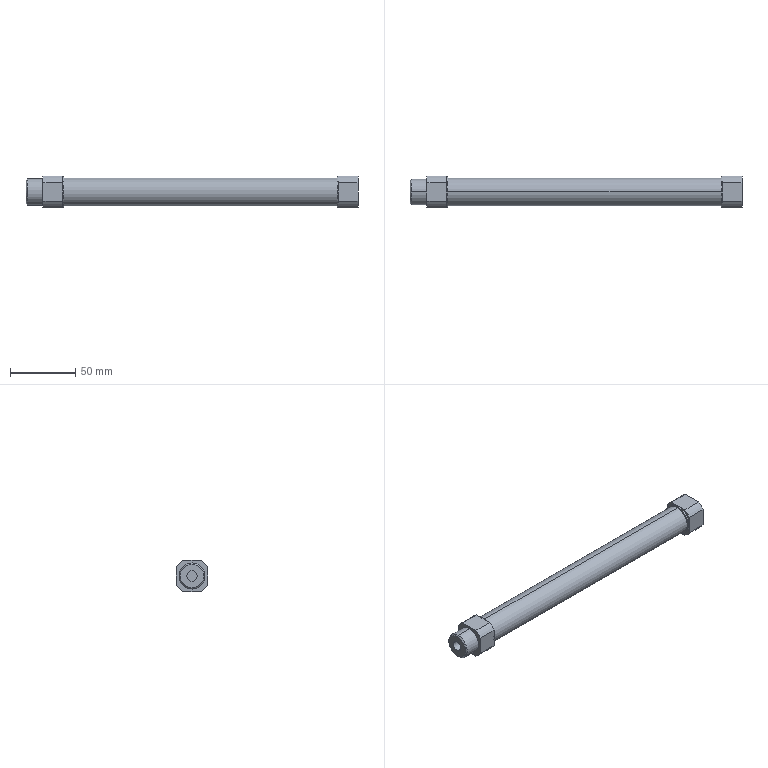Part | 1 solid | 60 faces | box 255 x 24 x 24 mm | volume 45614 mm3 | plane 28 | cylinder 26 | cone 6 | commonest cylinder face diameters 28 x8 8 x4 8.566 x4 24 x4 18 x2 20 x2